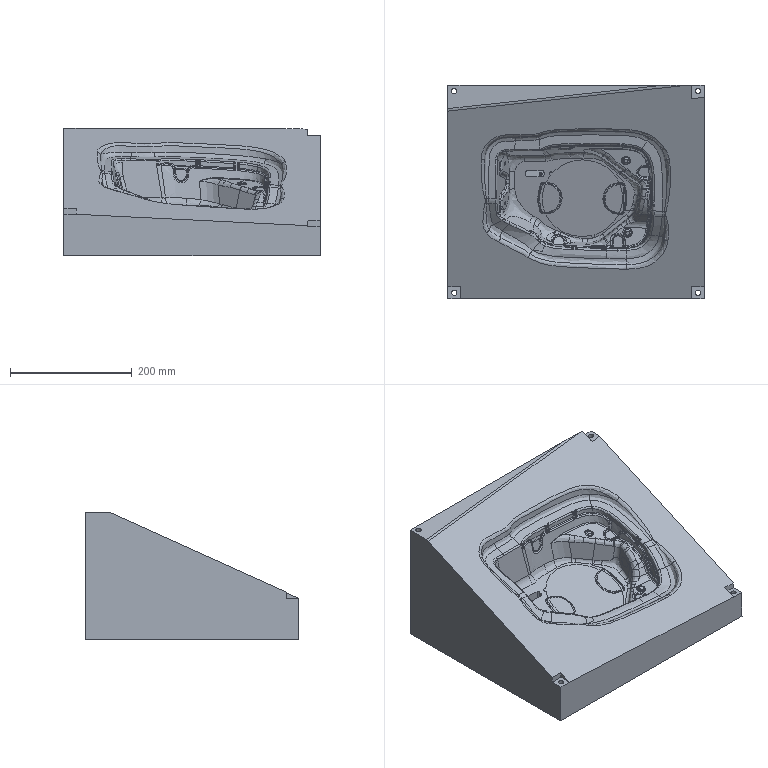NC program | NX | posted with a generic post | part box 420 x 350 x 208.3 mm
Lines 34642 to 35454 of 93858:
(CAVITY_MILL_COPY , TOOL : D16R0.8)
N69282 M6
N69284 G54
N69286 G17 G0 G90 X-106.492 Y82.897 S1900 M3
N69288 G43 Z220. H0
N69290 Z185.516
N69292 G94 G1 Z185.316 F3000.
N69294 X-106.56 Y84.36
N69296 G3 X-108.651 Y86.265 R2.
N69298 X-117.364 Y85.649 R179.786
N69300 X-122.973 Y84.713 R51.194
N69302 X-124.487 Y82.324 R2.
N69304 G1 X-124.166 Y80.895
N69306 Z185.516
N69308 G0 Z208.6
N69310 X-114.961 Y80.85
N69312 Z185.016
N69314 G1 Z184.816
N69316 X-115.155 Y82.841
N69318 G2 X-113.358 Y85.026 R2.
N69320 G1 X-98.528 Y86.472
N69322 G3 X-101.417 Y86.453 R1159.971
N69324 G1 X-101.971 Y86.393
N69326 G3 X-126.606 Y83.724 R576.071
N69328 G1 X-126.77 Y83.707
N69330 G3 X-128.153 Y83.261 R51.194
N69332 G1 X-121.49 Y84.138
N69334 X-118.387 Y84.531
N69336 G2 X-118.104 Y84.563 R9.883
N69338 G1 X-113.358 Y85.026
N69340 G2 X-111.174 Y83.229 R2.
N69342 G1 X-110.979 Y81.239
N69344 Z185.016
N69346 G0 Z185.616
N69348 X-114.926 Y80.207
N69350 Z184.516
N69352 G1 Z184.316
N69354 X-115.111 Y82.213
N69356 G2 X-113.303 Y84.387 R2.
N69358 G1 X-113.316 Y84.529
N69360 X-115.389 Y84.352
N69362 X-116.373 Y84.248
N69364 G3 X-130.684 Y82.176 R318.307
N69366 G1 X-130.794 Y82.164
N69368 G3 X-132.18 Y81.499 R42.315
N69370 G1 X-132.003 Y81.526
N69372 X-130.658 Y81.746
N69374 G3 X-130.3 Y81.813 R7.6
N69376 G2 X-127.265 Y82.426 R145.628
N69378 G3 X-126.905 Y82.485 R7.8
N69380 G2 X-109.621 Y84.679 R145.619
N69382 G3 X-100.963 Y85.288 R1140.22
N69384 G1 X-100.782 Y85.304
N69386 X-100.483 Y85.333
N69388 G3 X-86.376 Y86.473 R1140.211
N69390 X-90.885 Y86.488 R1159.971
N69392 G1 X-91.436 Y86.428
N69394 X-94.895 Y86.104
N69396 X-113.316 Y84.529
N69398 G3 X-115.138 Y82.366 R2.
N69400 G1 X-114.953 Y80.204
N69402 Z184.516
N69404 G0 Z185.116
N69406 X-114.911 Y79.631
N69408 Z184.017
N69410 G1 Z183.817
N69412 X-115.076 Y81.629
N69414 G2 X-113.248 Y83.787 R2.
N69416 G1 X-113.267 Y84.007
N69418 G3 X-123.262 Y82.721 R149.31
N69420 G1 X-132.12 Y80.987
N69422 X-133.528 Y80.762
N69424 X-133.594 Y80.755
N69426 G3 X-134.194 Y80.418 R42.315
N69428 G1 X-130.521 Y81.018
N69430 G3 X-130.162 Y81.086 R7.6
N69432 G2 X-127.987 Y81.532 R144.888
N69434 G3 X-127.654 Y81.605 R7.6
N69436 G2 X-126.146 Y81.959 R84.602
N69438 X-124.71 Y82.215 R144.963
N69440 G3 X-124.483 Y82.258 R7.8
N69442 G2 X-114.998 Y83.639 R84.546
N69444 X-100.419 Y84.672 R467.95
N69446 G1 X-100.267 Y84.682
N69448 G3 X-97.925 Y84.86 R1140.875
N69450 G2 X-97.476 Y84.882 R468.007
N69452 G3 X-95.582 Y84.97 R616.329
N69454 X-95.349 Y84.985 R7.6
N69456 X-77.921 Y86.498 R1140.951
N69458 G1 X-78.976 Y86.479
N69460 X-79.96 Y86.469
N69462 X-80.874 Y86.466
N69464 X-81.47 Y86.401
N69466 G2 X-107.516 Y84.439 R823.908
N69468 G3 X-113.267 Y84.007 R149.31
N69470 X-115.07 Y81.828 R2.
N69472 G1 X-114.862 Y79.635
N69474 Z184.017
N69476 G0 Z186.316
N69478 X-34.943 Y89.483
N69480 Z185.016
N69482 G1 Z184.816
N69484 X-35.159 Y91.473
N69486 G2 X-33.388 Y93.678 R2.
N69488 X-15.72 Y95.463 R1137.136
N69490 G1 X-16.974 Y95.426
N69492 X-19.222 Y95.357
N69494 X-20.023 Y95.27
N69496 G3 X-48.921 Y92.14 R994.453
N69498 G1 X-49.114 Y92.119
N69500 G3 X-51.025 Y91.618 R87.978
N69502 G2 X-33.388 Y93.678 R1137.136
N69504 X-31.183 Y91.906 R2.
N69506 G1 X-30.966 Y89.916
N69508 Z185.016
N69510 G0 Z185.616
N69512 X-34.896 Y88.78
N69514 Z184.516
N69516 G1 Z184.316
N69518 X-35.101 Y90.775
N69520 G2 X-33.316 Y92.969 R2.
N69522 G1 X-33.338 Y93.183
N69524 G3 X-49.45 Y91.162 R327.651
N69526 G1 X-50.278 Y91.016
N69528 X-50.434 Y90.994
N69530 X-51.418 Y90.865
N69532 X-54.925 Y90.383
N69534 X-55.239 Y90.349
N69536 G3 X-56.359 Y89.972 R87.978
N69538 G1 X-57.385 Y89.608
N69540 G3 X-49.513 Y90.854 R416.853
N69542 X-49.168 Y90.905 R7.8
N69544 X-46.069 Y91.441 R416.86
N69546 G2 X-45.633 Y91.509 R10.608
N69548 X-22.962 Y93.895 R397.074
N69550 G3 X-19.153 Y94.19 R1588.225
N69552 G1 X-19.019 Y94.202
N69554 G2 X-18.557 Y94.246 R1136.194
N69556 G3 X0.493 Y95.869 R1588.217
N69558 G1 X0.621 Y95.882
N69560 X0.733 Y95.894
N69562 G3 X-5.36 Y95.752 R1451.841
N69564 G1 X-6.074 Y95.675
N69566 G2 X-29.767 Y93.522 R2061.463
N69568 G3 X-33.338 Y93.183 R327.651
N69570 X-35.128 Y90.994 R2.
N69572 G1 X-34.906 Y88.779
N69574 Z184.516
N69576 G0 Z185.116
N69578 X-34.845 Y88.194
N69580 Z184.017
N69582 G1 Z183.817
N69584 X-35.046 Y90.191
N69586 G2 X-33.256 Y92.381 R2.
N69588 G1 X-33.278 Y92.595
N69590 G3 X-45.513 Y91.111 R322.299
N69592 G1 X-46.038 Y91.016
N69594 X-57.562 Y89.051
N69596 X-59.569 Y88.774
N69598 X-59.852 Y88.743
N69600 X-60.295 Y88.59
N69602 X-61.11 Y88.324
N69604 G3 X-52.631 Y89.594 R417.591
N69606 X-52.326 Y89.649 R7.6
N69608 G2 X-50.295 Y90.051 R243.892
N69610 G3 X-45.954 Y90.796 R417.516
N69612 G1 X-45.784 Y90.824
N69614 X-45.674 Y90.842
N69616 G2 X-44.513 Y91.041 R243.835
N69618 X-44.154 Y91.096 R11.087
N69620 X-26.455 Y92.993 R322.905
N69622 G1 X-24.904 Y93.113
N69624 X-24.81 Y93.12
N69626 X-21.713 Y93.333
N69628 G3 X-16.164 Y93.771 R1588.881
N69630 G1 X-10.681 Y94.147
N69632 X-10.565 Y94.156
N69634 G3 X10.463 Y96.066 R1588.957
N69636 X7.302 Y96.017 R1451.841
N69638 G1 X6.769 Y95.96
N69640 G2 X-23.862 Y93.415 R1233.165
N69642 G3 X-33.278 Y92.595 R322.299
N69644 X-35.065 Y90.402 R2.
N69646 G1 X-34.84 Y88.195
N69648 Z184.017
N69650 G0 Z184.616
N69652 X-34.811 Y87.737
N69654 Z183.517
N69656 G1 Z183.317
N69658 X-35.006 Y89.734
N69660 G2 X-33.211 Y91.92 R2.
N69662 G1 X-33.23 Y92.119
N69664 G3 X-44.529 Y90.758 R282.559
N69666 X-58.327 Y88.069 R477.561
N69668 G2 X-86.899 Y85.122 R318.175
N69670 G1 X-108.5 Y83.891
N69672 X-109.484 Y83.805
N69674 X-110.468 Y83.741
N69676 G3 X-122.278 Y82.409 R115.339
N69678 X-128.032 Y81.132 R89.611
N69680 G1 X-131.626 Y80.209
N69682 X-135.072 Y79.51
N69684 X-135.785 Y79.411
N69686 X-135.88 Y79.4
N69688 G3 X-136.843 Y78.77 R42.315
N69690 G1 X-136.71 Y78.784
N69692 G3 X-136.037 Y78.888 R7.6
N69694 X-132.287 Y79.788 R50.613
N69696 X-131.902 Y79.889 R7.8
N69698 X-131.659 Y79.96 R50.621
N69700 G2 X-123.166 Y82.024 R84.063
N69702 G1 X-123.048 Y82.048
N69704 G2 X-118.572 Y82.784 R58.328
N69706 G1 X-117.059 Y82.979
N69708 G2 X-116.628 Y83.027 R11.454
N69710 X-108.751 Y83.653 R356.783
N69712 X-97.452 Y84.343 R467.467
N69714 G3 X-78.609 Y85.482 R616.868
N69716 G1 X-78.469 Y85.494
N69718 G3 X-78.055 Y85.533 R1141.896
N69720 X-69.34 Y86.264 R616.86
N69722 X-60.126 Y87.505 R107.165
N69724 X-59.818 Y87.555 R7.8
N69726 X-56.089 Y88.304 R107.171
N69728 G2 X-44.433 Y90.565 R243.353
N69730 X-44.089 Y90.617 R10.604
N69732 G1 X-43.971 Y90.633
N69734 G3 X-43.707 Y90.673 R7.8
N69736 G2 X-42.981 Y90.795 R154.387
N69738 X-42.591 Y90.852 R11.454
N69740 X-27.285 Y92.442 R301.092
N69742 X-26.418 Y92.512 R322.422
N69744 G1 X-24.866 Y92.631
N69746 X-24.777 Y92.638
N69748 X4.15 Y94.626
N69750 G3 X8.845 Y94.96 R1014.068
N69752 G1 X9.024 Y94.975
N69754 G3 X9.309 Y95.002 R1589.903
N69756 X24.04 Y96.198 R1014.06
N69758 X18.86 Y96.163 R1451.841
N69760 G1 X18.29 Y96.101
N69762 G2 X-22.342 Y92.997 R1346.838
N69764 G3 X-33.23 Y92.119 R282.559
N69766 X-35.021 Y89.93 R2.
N69768 G1 X-34.802 Y87.738
N69770 Z183.517
N69772 G0 Z184.117
N69774 X-34.774 Y87.369
N69776 Z183.017
N69778 G1 Z182.817
N69780 X-34.969 Y89.366
N69782 G2 X-33.174 Y91.551 R2.
N69784 G1 X-33.19 Y91.715
N69786 G3 X-41.577 Y90.793 R415.625
N69788 X-53.387 Y88.506 R133.499
N69790 G2 X-68.149 Y85.891 R109.117
N69792 X-94.781 Y84.139 R481.858
N69794 G1 X-96.69 Y84.067
N69796 G3 X-114.405 Y83.044 R397.726
N69798 X-130.152 Y79.961 R67.378
N69800 G2 X-137.732 Y78.093 R47.579
N69802 G1 X-137.831 Y78.083
N69804 G3 X-138.307 Y77.737 R42.315
N69806 X-133.392 Y78.726 R51.355
N69808 X-132.849 Y78.884 R7.6
N69810 G1 X-131.801 Y79.234
N69812 G3 X-131.472 Y79.33 R51.279
N69814 G2 X-130.62 Y79.579 R83.405
N69816 G3 X-130.288 Y79.683 R7.8
N69818 G1 X-129.995 Y79.782
N69820 G2 X-120.387 Y82.154 R57.958
N69822 X-117.453 Y82.557 R50.687
N69824 G1 X-117.289 Y82.576
N69826 X-117.012 Y82.612
N69828 G2 X-116.594 Y82.658 R11.084
N69830 X-113.785 Y82.901 R356.412
N69832 X-111.108 Y83.113 R210.571
N69834 X-95.782 Y83.933 R356.412
N69836 G3 X-82.886 Y84.515 R680.019
N69838 G1 X-82.775 Y84.522
N69840 G3 X-78.957 Y84.797 R617.526
N69842 X-73.975 Y85.116 R679.963
N69844 G1 X-73.857 Y85.125
N69846 G3 X-69.273 Y85.525 R617.602
N69848 X-62.554 Y86.35 R107.904
N69850 G1 X-62.416 Y86.373
N69852 G3 X-58.965 Y87.045 R85.941
N69854 X-57.119 Y87.412 R107.828
N69856 X-56.869 Y87.468 R7.8
N69858 X-56.232 Y87.625 R85.997
N69860 G2 X-42.92 Y90.429 R154.016
N69862 X-42.543 Y90.485 R11.084
N69864 X-23.152 Y92.364 R300.722
N69866 G1 X-20.045 Y92.548
N69868 X4.711 Y94.006
N69870 G3 X9.135 Y94.322 R1014.725
N69872 G1 X13.553 Y94.582
N69874 X13.698 Y94.592
N69876 G3 X32.287 Y96.217 R1014.802
N69878 X29.561 Y96.216 R1451.841
N69880 G1 X29.001 Y96.155
N69882 G2 X-0.65 Y93.884 R928.909
N69884 G1 X-26.814 Y92.301
N69886 G3 X-33.19 Y91.715 R415.625
N69888 X-34.982 Y89.526 R2.
N69890 G1 X-34.767 Y87.369
N69892 Z183.017
N69894 G0 Z183.617
N69896 X-34.742 Y87.078
N69898 Z182.518
N69900 G1 Z182.318
N69902 X-34.939 Y89.075
N69904 G2 X-33.146 Y91.262 R2.
N69906 G1 X-33.16 Y91.411
N69908 G3 X-43.545 Y90.173 R246.484
N69910 X-55.355 Y87.552 R147.029
N69912 G2 X-66.181 Y85.451 R86.786
N69914 X-89.834 Y83.91 R321.227
N69916 G3 X-110.468 Y83.031 R719.048
N69918 X-117.731 Y82.386 R137.776
N69920 X-128.883 Y79.865 R53.391
N69922 G1 X-134.088 Y78.084
N69924 X-135.072 Y77.782
N69926 G2 X-139.436 Y76.802 R24.42
N69928 G1 X-139.54 Y76.791
N69930 G3 X-140.031 Y76.394 R42.315
N69932 X-140.295 Y76.175 R44.111
N69934 G1 X-139.804 Y76.228
N69936 G3 X-138.768 Y76.414 R7.6
N69938 X-137.226 Y76.864 R21.324
N69940 G1 X-136.442 Y77.126
N69942 G3 X-136.101 Y77.231 R7.8
N69944 G1 X-131.362 Y78.811
N69946 X-129.839 Y79.323
N69948 G2 X-129.603 Y79.403 R57.473
N69950 G3 X-129.392 Y79.477 R7.8
N69952 G2 X-126.266 Y80.51 R50.402
N69954 G1 X-126.135 Y80.546
N69956 G2 X-116.663 Y82.348 R50.401
N69958 X-103.594 Y83.236 R210.285
N69960 G1 X-101.975 Y83.294
N69962 X-101.82 Y83.301
N69964 X-85.645 Y83.886
N69966 X-85.532 Y83.891
N69968 G3 X-71.309 Y84.761 R680.503
N69970 X-56.113 Y87.156 R86.481
N69972 G2 X-54.952 Y87.45 R153.532
N69974 X-51.788 Y88.264 R4996.952
N69976 X-50.462 Y88.596 R101.324
N69978 G1 X-50.325 Y88.628
N69980 G2 X-42.971 Y90.116 R101.322
N69982 X-42.619 Y90.168 R11.451
N69984 X-26.46 Y91.843 R287.503
N69986 X-26.218 Y91.859 R11.451
N69988 G1 X-13.651 Y92.537
N69990 X-13.399 Y92.551
N69992 X1.711 Y93.366
N69994 X1.865 Y93.373
N69996 X2.921 Y93.416
N69998 X3.064 Y93.423
N70000 X18.446 Y94.329
N70002 X32.753 Y95.309
N70004 G3 X32.975 Y95.328 R7.8
N70006 G1 X33.148 Y95.345
N70008 X36.752 Y95.592
N70010 G3 X44.043 Y96.146 R486.24
N70012 G1 X44.193 Y96.16
N70014 G3 X39.571 Y96.194 R1451.841
N70016 G1 X39.04 Y96.136
N70018 G2 X12.584 Y94.161 R688.856
N70020 G1 X-19.925 Y92.363
N70022 X-23.862 Y92.143
N70024 G3 X-33.16 Y91.411 R246.484
N70026 X-34.956 Y89.226 R2.
N70028 G1 X-34.746 Y87.077
N70030 Z182.518
N70032 G0 Z183.117
N70034 X-34.728 Y86.805
N70036 Z182.018
N70038 G1 Z181.818
N70040 X-34.919 Y88.804
N70042 G2 X-33.118 Y90.985 R2.
N70044 G1 X-33.132 Y91.132
N70046 G3 X-34.688 Y90.968 R194.465
N70048 X-43.545 Y89.885 R158.529
N70050 X-55.552 Y87.087 R127.859
N70052 G2 X-69.133 Y84.61 R70.304
N70054 X-86.848 Y83.633 R326.915
N70056 G3 X-109.484 Y82.822 R956.818
N70058 X-117.357 Y82.164 R138.495
N70060 X-129.477 Y79.227 R47.278
N70062 G1 X-135.072 Y77.076
N70064 X-136.057 Y76.735
N70066 G2 X-140.957 Y75.531 R23.284
N70068 G1 X-141.059 Y75.52
N70070 G3 X-141.454 Y75.169 R44.111
N70072 X-136.991 Y76.158 R22.068
N70074 G1 X-136.126 Y76.447
N70076 G3 X-135.666 Y76.617 R7.6
N70078 G1 X-134.788 Y76.974
N70080 X-134.208 Y77.167
N70082 G3 X-133.736 Y77.342 R7.8
N70084 G1 X-130.881 Y78.503
N70086 G2 X-128.293 Y79.474 R50.031
N70088 G3 X-128.002 Y79.58 R7.8
N70090 G2 X-127.535 Y79.76 R79.198
N70092 X-127.326 Y79.837 R11.736
N70094 X-125.453 Y80.398 R50.071
N70096 G1 X-125.356 Y80.426
N70098 G2 X-116.719 Y82.093 R47.08
N70100 X-101.93 Y82.993 R208.302
N70102 G3 X-98.428 Y83.093 R18362.944
N70104 G1 X-93.698 Y83.264
N70106 G3 X-87.891 Y83.433 R18362.913
N70108 G1 X-82.201 Y83.639
N70110 G3 X-67.883 Y84.554 R258.855
N70112 X-58.082 Y86.259 R61.716
N70114 G2 X-54.355 Y87.221 R4996.58
N70116 G1 X-54.235 Y87.253
N70118 X-51.894 Y87.896
N70120 X-51.706 Y87.944
N70122 G2 X-49.548 Y88.474 R100.993
N70124 X-40.112 Y90.216 R81.642
N70126 X-21.458 Y91.822 R246.932
N70128 G1 X-18.364 Y91.957
N70130 X-17.515 Y91.998
N70132 X-11.136 Y92.342
N70134 X-3.649 Y92.706
N70136 X1.731 Y92.996
N70138 X1.88 Y93.003
N70140 X3.416 Y93.065
N70142 X26.053 Y94.191
N70144 X26.198 Y94.2
N70146 X29.092 Y94.398
N70148 X33.127 Y94.599
N70150 X33.269 Y94.607
N70152 X36.803 Y94.849
N70154 G3 X51.476 Y96.078 R486.984
N70156 X49.01 Y96.11 R1451.841
N70158 G1 X48.496 Y96.054
N70160 G2 X18.165 Y93.964 R689.188
N70162 G3 X-23.49 Y91.87 R16386.454
N70164 X-33.132 Y91.132 R194.465
N70166 X-34.92 Y88.94 R2.
N70168 G1 X-34.703 Y86.808
N70170 Z182.018
N70172 G0 Z182.618
N70174 X-34.7 Y86.581
N70176 Z181.518
N70178 G1 Z181.318
N70180 X-34.894 Y88.581
N70182 G2 X-33.097 Y90.765 R2.
N70184 G1 X-33.112 Y90.923
N70186 G3 X-41.478 Y89.972 R241.713
N70188 X-48.237 Y88.689 R60.371
N70190 G1 X-48.466 Y88.632
N70192 X-49.45 Y88.409
N70194 X-50.434 Y88.141
N70196 X-50.694 Y88.069
N70198 G3 X-56.339 Y86.523 R255.09
N70200 G2 X-68.736 Y84.22 R62.115
N70202 X-84.448 Y83.38 R275.356
N70204 G3 X-104.563 Y82.819 R3335.508
N70206 X-116.373 Y82.073 R199.845
N70208 X-125.231 Y80.386 R49.093
N70210 X-130.369 Y78.483 R56.561
N70212 G1 X-136.057 Y76.057
N70214 X-137.429 Y75.529
N70216 G2 X-142.34 Y74.275 R21.738
N70218 G1 X-142.431 Y74.265
N70220 G3 X-143.057 Y73.655 R44.111
N70222 G1 X-142.962 Y73.665
N70224 G3 X-142.091 Y73.811 R7.6
N70226 X-139.369 Y74.583 R27.205
N70228 X-138.978 Y74.711 R7.8
N70230 X-138.207 Y75. R27.213
N70232 G1 X-138.114 Y75.037
N70234 X-133.239 Y77.02
N70236 G3 X-132.86 Y77.186 R7.8
N70238 G2 X-130.818 Y78.11 R78.912
N70240 G1 X-130.704 Y78.159
N70242 G2 X-127.433 Y79.492 R78.911
N70244 X-126.973 Y79.656 R11.449
N70246 X-124.834 Y80.313 R46.827
N70248 G1 X-124.7 Y80.352
N70250 G2 X-118.683 Y81.633 R37.581
N70252 X-111.985 Y82.297 R90.589
N70254 X-104.788 Y82.648 R282.183
N70256 X-101.923 Y82.74 R208.05
N70258 G3 X-80.248 Y83.372 R18363.203
N70260 X-76.331 Y83.53 R199.763
N70262 X-68.495 Y84.075 R199.762
N70264 X-60.101 Y85.376 R64.15
N70266 X-59.558 Y85.499 R62.103
N70268 X-59.255 Y85.576 R7.941
N70270 G1 X-51.593 Y87.681
N70272 G2 X-46.685 Y88.867 R81.39
N70274 X-37.652 Y90.295 R80.814
N70276 G1 X-36.127 Y90.449
N70278 G2 X-20.274 Y91.627 R217.588
N70280 G1 X-19.858 Y91.642
N70282 G2 X-16.52 Y91.794 R3212.458
N70284 G1 X1.859 Y92.685
N70286 X11.68 Y93.088
N70288 X22.811 Y93.544
N70290 X38.615 Y94.331
N70292 X51.203 Y95.097
N70294 G3 X51.556 Y95.126 R7.8
N70296 X62.176 Y95.895 R487.015
N70298 X57.983 Y95.975 R786.793
N70300 G1 X57.475 Y95.92
N70302 G2 X27.881 Y93.964 R657.856
N70304 G3 X-18.941 Y91.859 R14024.414
N70306 G1 X-19.925 Y91.813
N70308 X-20.909 Y91.784
N70310 G3 X-33.112 Y90.923 R241.713
N70312 X-34.912 Y88.741 R2.
N70314 G1 X-34.704 Y86.581
N70316 Z181.518
N70318 G0 Z182.118
N70320 X-34.696 Y86.429
N70322 Z181.019
N70324 G1 Z180.819
N70326 X-34.885 Y88.43
N70328 G2 X-33.082 Y90.61 R2.
N70330 G1 X-33.096 Y90.753
N70332 G3 X-37.64 Y90.265 R205.469
N70334 G1 X-37.971 Y90.232
N70336 G3 X-50.188 Y87.979 R74.835
N70338 X-56.738 Y86.104 R254.601
N70340 G2 X-68.149 Y83.934 R56.168
N70342 X-79.959 Y83.223 R199.533
N70344 X-97.674 Y82.821 R1221.439
N70346 G3 X-111.452 Y82.311 R402.115
N70348 X-118.342 Y81.665 R96.239
N70350 X-130.152 Y78.22 R39.426
N70352 G1 X-137.041 Y75.022
N70354 G2 X-143.681 Y73.023 R23.179
N70356 G3 X-143.997 Y72.693 R44.111
N70358 X-139.384 Y73.791 R27.951
N70360 X-138.649 Y74.076 R7.6
N70362 X-137.96 Y74.387 R117.743
N70364 G1 X-137.869 Y74.423
N70366 X-137.099 Y74.737
N70368 G3 X-136.715 Y74.905 R7.8
N70370 X-134.493 Y75.98 R117.797
N70372 G2 X-131.736 Y77.296 R78.54
N70374 G3 X-131.468 Y77.423 R7.8
N70376 G2 X-130.75 Y77.779 R107.243
N70378 X-130.212 Y78.012 R78.581
N70380 G3 X-129.915 Y78.146 R7.941
N70382 G2 X-122.77 Y80.684 R37.394
N70384 X-118.682 Y81.472 R34.569
N70386 X-108.257 Y82.322 R111.404
N70388 X-107.353 Y82.357 R617.606
N70390 X-102.063 Y82.546 R281.995
N70392 G1 X-97.206 Y82.674
N70394 X-86.35 Y82.889
N70396 X-82.417 Y82.977
N70398 G3 X-80.238 Y83.042 R18363.524
N70400 X-69.797 Y83.631 R200.093
N70402 X-68.421 Y83.741 R229.538
N70404 X-62.14 Y84.618 R56.414
N70406 X-59.476 Y85.18 R64.481
N70408 X-59.174 Y85.256 R7.941
N70410 G1 X-57.404 Y85.743
N70412 G3 X-57.162 Y85.813 R7.941
N70414 G1 X-56.985 Y85.868
N70416 X-56.82 Y85.917
N70418 X-52.378 Y87.219
N70420 G2 X-47.004 Y88.605 R80.626
N70422 G1 X-46.899 Y88.629
N70424 G2 X-41.288 Y89.667 R58.749
N70426 X-23.897 Y91.272 R206.251
N70428 X-20.267 Y91.439 R217.401
N70430 G1 X-19.85 Y91.455
N70432 G2 X9.772 Y92.679 R3212.269
N70434 G1 X16.307 Y92.946
N70436 G2 X22.028 Y93.14 R3212.303
N70438 G1 X46.06 Y94.123
N70440 X46.215 Y94.131
N70442 X49.097 Y94.307
N70444 X53.828 Y94.525
N70446 X53.981 Y94.533
N70448 G3 X68.635 Y95.727 R487.762
N70450 X66.476 Y95.789 R786.793
N70452 G1 X66.052 Y95.743
N70454 G2 X47.549 Y94.422 R420.703
N70456 G1 X38.242 Y93.964
N70458 G2 X4.679 Y92.667 R5477.318
N70460 X-2.21 Y92.376 R374.168
N70462 G1 X-22.878 Y91.479
N70464 G3 X-33.096 Y90.753 R205.469
N70466 X-34.895 Y88.571 R2.
N70468 G1 X-34.689 Y86.43
N70470 Z181.019
N70472 G0 Z181.618
N70474 X-34.683 Y86.302
N70476 Z180.519
N70478 G1 Z180.319
N70480 X-34.872 Y88.303
N70482 G2 X-33.07 Y90.482 R2.
N70484 G1 X-33.082 Y90.611
N70486 G3 X-39.608 Y89.909 R289.538
N70488 X-49.171 Y88.069 R64.886
N70490 X-56.339 Y85.975 R219.444
N70492 G2 X-61.26 Y84.65 R69.502
N70494 X-72.086 Y83.344 R70.712
N70496 X-77.991 Y83.034 R109.815
N70498 X-100.627 Y82.588 R1603.082
N70500 G3 X-115.389 Y81.883 R236.178
N70502 X-123.262 Y80.577 R48.578
N70504 X-131.488 Y77.262 R42.451
N70506 G2 X-139.009 Y73.507 R180.967
N70508 X-144.826 Y71.793 R20.309
N70510 G3 X-145.362 Y71.184 R44.111
N70512 G1 X-145.277 Y71.193
N70514 G3 X-144.289 Y71.367 R7.6
N70516 X-141.439 Y72.287 R20.681
N70518 X-141.1 Y72.42 R7.8
N70520 X-136.059 Y74.678 R118.284
N70522 X-135.612 Y74.909 R7.8
N70524 G2 X-133.914 Y75.836 R106.956
N70526 G1 X-133.816 Y75.887
N70528 G2 X-129.807 Y77.918 R106.956
N70530 X-129.066 Y78.259 R37.14
N70532 G1 X-128.914 Y78.329
N70534 G2 X-120.951 Y80.965 R34.439
N70536 X-119.867 Y81.17 R32.302
N70538 X-115.075 Y81.785 R57.531
N70540 G1 X-114.973 Y81.793
N70542 G2 X-111.914 Y82.006 R199.462
N70544 X-109.065 Y82.161 R111.274
N70546 X-104.31 Y82.331 R199.462
N70548 X-89.275 Y82.627 R617.476
N70550 G3 X-79.558 Y82.804 R369.016
N70552 X-68.397 Y83.454 R229.825
N70554 X-57.689 Y85.388 R56.701
N70556 G1 X-57.499 Y85.444
N70558 X-56.91 Y85.626
N70560 X-56.749 Y85.675
N70562 X-56.54 Y85.736
N70564 X-56.367 Y85.789
N70566 G2 X-48.883 Y87.99 R177.783
N70568 X-41.271 Y89.539 R58.619
N70570 X-40.849 Y89.595 R206.121
N70572 X-40.276 Y89.673 R64.716
N70574 X-24.7 Y91.104 R206.811
N70576 X-24.43 Y91.116 R12.092
N70578 G1 X-24.32 Y91.121
N70580 G2 X-22.13 Y91.222 R206.121
N70582 X8.07 Y92.363 R4496.663
N70584 X32.504 Y93.18 R3212.017
N70586 X33.035 Y93.196 R3212.016
N70588 G3 X41.127 Y93.435 R3494.821
N70590 G1 X48.435 Y93.734
N70592 X60.008 Y94.267
N70594 G3 X67.625 Y94.672 R536.603
N70596 X67.974 Y94.701 R7.8
N70598 X77.859 Y95.395 R536.596
N70600 X74.34 Y95.534 R786.793
N70602 G1 X74.09 Y95.507
N70604 G2 X49.487 Y93.964 R451.648
N70606 X11.359 Y92.634 R5659.818
N70608 G3 X-12.052 Y91.76 R1999.775
N70610 X-26.814 Y91.146 R1021.287
N70612 X-33.082 Y90.611 R289.538
N70614 X-34.881 Y88.429 R2.
N70616 G1 X-34.677 Y86.303
N70618 Z180.519
N70620 G0 Z181.119
N70622 X-34.676 Y86.225
N70624 Z180.019
N70626 G1 Z179.819
N70628 X-34.865 Y88.226
N70630 G2 X-33.063 Y90.406 R2.
N70632 G1 X-33.075 Y90.532
N70634 G3 X-41.577 Y89.553 R201.035
N70636 X-48.639 Y88.069 R56.399
N70638 X-56.339 Y85.759 R143.072
N70640 G2 X-66.181 Y83.612 R53.86
N70642 X-75.038 Y82.934 R124.598
N70644 X-88.817 Y82.607 R377.412
N70646 G3 X-103.579 Y82.4 R1303.245
N70648 X-113.421 Y81.972 R229.923
N70650 X-119.516 Y81.279 R63.446
N70652 X-129.675 Y77.917 R33.976
N70654 G1 X-131.136 Y77.161
N70656 X-136.668 Y74.089
N70658 G2 X-141.046 Y71.92 R52.242
N70660 X-145.881 Y70.572 R17.831
N70662 G3 X-146.151 Y70.244 R44.111
N70664 X-141.055 Y71.636 R21.43
N70666 G1 X-140.872 Y71.712
N70668 G3 X-140.368 Y71.946 R7.6
N70670 X-139.61 Y72.336 R83.475
N70672 X-139.203 Y72.514 R118.945
N70674 X-138.637 Y72.789 R7.8
N70676 X-136.622 Y73.908 R83.53
N70678 G2 X-134.783 Y74.942 R106.584
N70680 G3 X-134.536 Y75.083 R7.8
N70682 G2 X-133.738 Y75.555 R89.321
N70684 X-133.028 Y75.93 R106.625
N70686 G3 X-132.797 Y76.056 R7.941
N70688 G2 X-130.382 Y77.378 R89.287
N70690 X-128.583 Y78.277 R34.251
N70692 G1 X-128.459 Y78.335
N70694 G2 X-119.854 Y81.094 R32.225
N70696 X-115.068 Y81.708 R57.454
N70698 G1 X-114.967 Y81.716
N70700 G2 X-114.469 Y81.754 R199.385
N70702 G1 X-114.373 Y81.762
N70704 G2 X-111.504 Y81.96 R80.695
N70706 X-111.043 Y81.981 R368.612
N70708 G1 X-110.952 Y81.986
N70710 G2 X-103.41 Y82.273 R199.385
N70712 X-86.164 Y82.482 R1199.417
N70714 G3 X-84.485 Y82.494 R287.41
N70716 X-74.236 Y82.821 R369.203
N70718 X-67.13 Y83.355 R125.631
N70720 X-57.335 Y85.294 R53.327
N70722 X-57.141 Y85.354 R7.941
N70724 G2 X-50.022 Y87.551 R240.686
N70726 X-42.096 Y89.331 R64.639
N70728 X-38.978 Y89.76 R62.483
N70730 X-24.696 Y91.027 R206.734
N70732 G1 X-24.504 Y91.036
N70734 G2 X3.559 Y92.039 R6782.361
N70736 X5.973 Y92.102 R3690.103
N70738 X9.758 Y92.233 R4496.475
N70740 X30.217 Y92.78 R8380.025
N70742 X33.044 Y92.865 R3211.686
N70744 G3 X38.174 Y93.014 R3495.152
N70746 G2 X44.527 Y93.168 R8380.062
N70748 G3 X65.926 Y93.911 R3495.193
N70750 G1 X66.078 Y93.918
N70752 G3 X68.574 Y94.067 R537.265
N70754 X71.513 Y94.181 R3495.137
N70756 X71.729 Y94.193 R7.6
N70758 X83.183 Y95.094 R537.344
N70760 X81.532 Y95.207 R172.4
N70762 G1 X81.189 Y95.17
N70764 G2 X48.966 Y93.48 R676.284
N70766 G1 X9.6 Y92.376
N70768 X3.695 Y92.195
N70770 G3 X-23.862 Y91.182 R6195.547
N70772 X-33.075 Y90.532 R201.035
N70774 X-34.879 Y88.354 R2.
N70776 G1 X-34.68 Y86.225
N70778 Z180.019
N70780 G0 Z180.619
N70782 X-34.67 Y86.167
N70784 Z179.52
N70786 G1 Z179.32
N70788 X-34.86 Y88.168
N70790 G2 X-33.057 Y90.347 R2.
N70792 G1 X-33.069 Y90.475
N70794 G3 X-37.64 Y89.982 R184.105
N70796 G1 X-37.928 Y89.956
N70798 G3 X-49.515 Y87.735 R61.262
N70800 X-56.339 Y85.61 R222.68
N70802 G2 X-68.59 Y83.157 R51.715
N70804 X-79.959 Y82.596 R177.246
N70806 X-96.69 Y82.432 R1069.021
N70808 G3 X-110.468 Y82.095 R347.117
N70810 X-118.342 Y81.42 R93.083
N70812 G1 X-121.294 Y80.896
N70814 G3 X-129.167 Y77.976 R31.767
N70816 X-135.072 Y74.58 R100.743
N70818 G2 X-140.977 Y71.23 R85.477
N70820 X-146.853 Y69.36 R18.436
N70822 G3 X-147.317 Y68.751 R44.111
N70824 G1 X-147.24 Y68.759
N70826 G3 X-146.21 Y68.943 R7.6
N70828 X-143.281 Y69.947 R18.298
N70830 X-142.95 Y70.091 R7.8
N70832 X-138.15 Y72.499 R84.017
N70834 X-137.646 Y72.797 R7.8
N70836 X-137.021 Y73.202 R108.649
N70838 G2 X-136.488 Y73.544 R89.034
N70840 G1 X-136.411 Y73.592
N70842 G2 X-131.958 Y76.237 R89.033
N70844 G3 X-131.687 Y76.395 R7.941
N70846 G2 X-130.859 Y76.893 R112.641
N70848 X-127.5 Y78.637 R32.095
N70850 G1 X-127.358 Y78.703
N70852 G2 X-123.941 Y80.055 R29.3
N70854 X-119.844 Y81.036 R32.166
N70856 X-115.063 Y81.65 R57.395
N70858 G1 X-114.963 Y81.658
N70860 G2 X-114.465 Y81.696 R199.326
N70862 G1 X-114.368 Y81.703
N70864 G2 X-111.501 Y81.901 R80.636
N70866 X-111.041 Y81.923 R368.553
N70868 G1 X-110.949 Y81.927
N70870 G2 X-103.409 Y82.214 R199.326
N70872 X-96.438 Y82.329 R1199.358
N70874 X-91.892 Y82.327 R368.586
N70876 G3 X-90.73 Y82.321 R419.572
N70878 G1 X-90.631
N70880 G2 X-86.163 Y82.352 R1199.286
N70882 G3 X-71.688 Y82.777 R287.541
N70884 X-65.649 Y83.332 R81.974
N70886 X-57.138 Y85.218 R48.77
N70888 G2 X-53.539 Y86.359 R240.555
N70890 G1 X-53.44 Y86.391
N70892 G2 X-50.952 Y87.188 R540.082
N70894 X-48.14 Y88.009 R62.456
N70896 X-42.087 Y89.273 R64.581
N70898 X-38.97 Y89.702 R62.425
N70900 X-24.693 Y90.968 R206.676